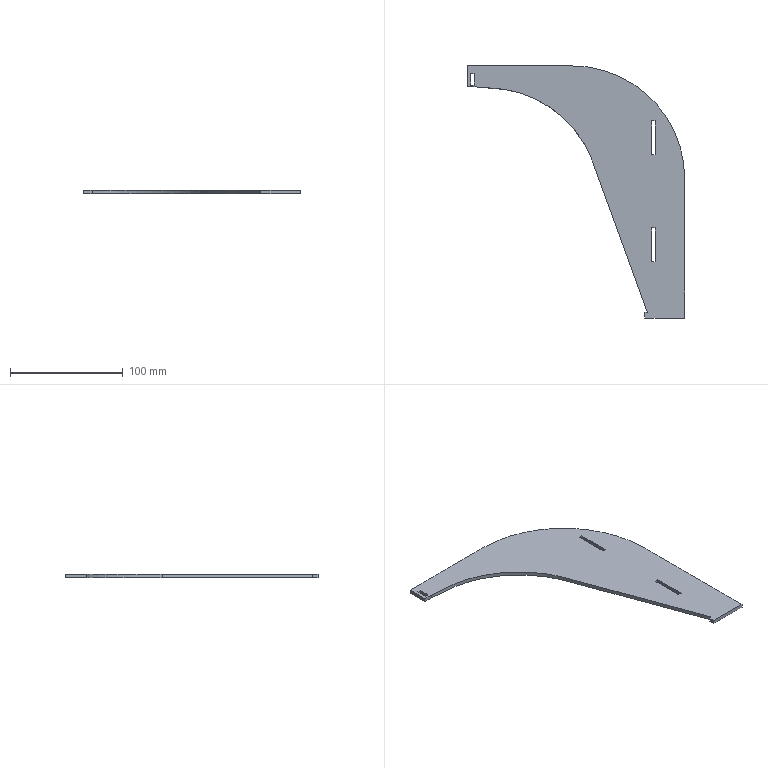Part | SolidWorks | features FlatPattern 1, SMBaseFlange 1, SheetMetal 1 | 1 solid | 24 faces | box 192.85 x 223.811 x 3.2 mm | volume 52018 mm3 | plane 22 | spline 1 | cylinder 1 | commonest cylinder face diameters 200 x1
STEP:
#1=CARTESIAN_POINT('',(111.323,-0.6438,0.));
#2=VERTEX_POINT('',#1);
#3=CARTESIAN_POINT('',(159.825,-133.885,0.));
#4=VERTEX_POINT('',#3);
#5=CARTESIAN_POINT('',(111.323,-0.6438,0.));
#6=CARTESIAN_POINT('',(127.491,-45.057,0.));
#7=CARTESIAN_POINT('',(143.658,-89.471,0.));
#8=CARTESIAN_POINT('',(159.825,-133.885,0.));
#9=B_SPLINE_CURVE_WITH_KNOTS('',3,(#5,#6,#7,#8),.UNSPECIFIED.,.F.,.F.,(4,4),(0.,1.),.UNSPECIFIED.);
#10=EDGE_CURVE('',#2,#4,#9,.T.);
#11=ORIENTED_EDGE('',*,*,#10,.F.);
#12=CARTESIAN_POINT('',(111.323,-0.6438,-3.2));
#13=VERTEX_POINT('',#12);
#14=CARTESIAN_POINT('',(111.323,-0.6438,-3.2));
#15=DIRECTION('',(0.,0.,1.));
#16=VECTOR('',#15,1000.);
#17=LINE('',#14,#16);
#18=EDGE_CURVE('',#13,#2,#17,.T.);
#19=ORIENTED_EDGE('',*,*,#18,.F.);
#20=CARTESIAN_POINT('',(159.825,-133.885,-3.2));
#21=VERTEX_POINT('',#20);
#22=CARTESIAN_POINT('',(111.323,-0.6438,-3.2));
#23=CARTESIAN_POINT('',(127.491,-45.057,-3.2));
#24=CARTESIAN_POINT('',(143.658,-89.471,-3.2));
#25=CARTESIAN_POINT('',(159.825,-133.885,-3.2));
#26=B_SPLINE_CURVE_WITH_KNOTS('',3,(#22,#23,#24,#25),.UNSPECIFIED.,.F.,.F.,(4,4),(0.,1.),.UNSPECIFIED.);
#27=EDGE_CURVE('',#13,#21,#26,.T.);
#28=ORIENTED_EDGE('',*,*,#27,.T.);
#29=CARTESIAN_POINT('',(159.825,-133.885,-3.2));
#30=DIRECTION('',(0.,0.,1.));
#31=VECTOR('',#30,1000.);
#32=LINE('',#29,#31);
#33=EDGE_CURVE('',#21,#4,#32,.T.);
#34=ORIENTED_EDGE('',*,*,#33,.T.);
#35=EDGE_LOOP('',(#11,#19,#28,#34));
#36=FACE_OUTER_BOUND('',#35,.T.);
#37=CARTESIAN_POINT('',(111.323,-0.6438,-3.2));
#38=DIRECTION('',(-0.9397,-0.3421,0.));
#39=DIRECTION('',(0.3421,-0.9397,0.));
#40=AXIS2_PLACEMENT_3D('',#37,#38,#39);
#41=PLANE('',#40);
#42=ADVANCED_FACE('',(#36),#41,.T.);
#43=CARTESIAN_POINT('',(7.851,66.042,0.));
#44=VERTEX_POINT('',#43);
#45=CARTESIAN_POINT('',(7.851,66.042,0.));
#46=CARTESIAN_POINT('',(9.365,65.953,0.));
#47=CARTESIAN_POINT('',(11.527,65.821,0.));
#48=CARTESIAN_POINT('',(13.859,65.666,0.));
#49=CARTESIAN_POINT('',(14.977,65.589,0.));
#50=CARTESIAN_POINT('',(15.525,65.55,0.));
#51=CARTESIAN_POINT('',(15.795,65.531,0.));
#52=CARTESIAN_POINT('',(15.93,65.521,0.));
#53=CARTESIAN_POINT('',(15.987,65.517,0.));
#54=CARTESIAN_POINT('',(16.026,65.514,0.));
#55=CARTESIAN_POINT('',(16.043,65.513,0.));
#56=CARTESIAN_POINT('',(17.399,65.415,0.));
#57=CARTESIAN_POINT('',(19.426,65.26,0.));
#58=CARTESIAN_POINT('',(21.833,65.063,0.));
#59=CARTESIAN_POINT('',(23.047,64.961,0.));
#60=CARTESIAN_POINT('',(23.657,64.908,0.));
#61=CARTESIAN_POINT('',(23.962,64.882,0.));
#62=CARTESIAN_POINT('',(24.115,64.868,0.));
#63=CARTESIAN_POINT('',(24.192,64.862,0.));
#64=CARTESIAN_POINT('',(24.23,64.858,0.));
#65=CARTESIAN_POINT('',(24.246,64.857,0.));
#66=CARTESIAN_POINT('',(24.257,64.856,0.));
#67=CARTESIAN_POINT('',(24.261,64.855,0.));
#68=CARTESIAN_POINT('',(25.155,64.777,0.));
#69=CARTESIAN_POINT('',(26.332,64.671,0.));
#70=CARTESIAN_POINT('',(27.438,64.563,0.));
#71=CARTESIAN_POINT('',(27.924,64.514,0.));
#72=CARTESIAN_POINT('',(28.15,64.49,0.));
#73=CARTESIAN_POINT('',(28.259,64.479,0.));
#74=CARTESIAN_POINT('',(28.312,64.473,0.));
#75=CARTESIAN_POINT('',(28.339,64.47,0.));
#76=CARTESIAN_POINT('',(28.35,64.469,0.));
#77=CARTESIAN_POINT('',(28.358,64.468,0.));
#78=CARTESIAN_POINT('',(28.36,64.468,0.));
#79=CARTESIAN_POINT('',(29.048,64.393,0.));
#80=CARTESIAN_POINT('',(30.071,64.272,0.));
#81=CARTESIAN_POINT('',(31.26,64.112,0.));
#82=CARTESIAN_POINT('',(31.769,64.039,0.));
#83=CARTESIAN_POINT('',(32.107,63.989,0.));
#84=CARTESIAN_POINT('',(32.276,63.964,0.));
#85=CARTESIAN_POINT('',(33.809,63.733,0.));
#86=CARTESIAN_POINT('',(35.841,63.383,0.));
#87=CARTESIAN_POINT('',(38.19,62.903,0.));
#88=CARTESIAN_POINT('',(39.192,62.682,0.));
#89=CARTESIAN_POINT('',(39.859,62.532,0.));
#90=CARTESIAN_POINT('',(40.19,62.455,0.));
#91=CARTESIAN_POINT('',(43.202,61.742,0.));
#92=CARTESIAN_POINT('',(45.843,61.001,0.));
#93=CARTESIAN_POINT('',(51.055,59.304,0.));
#94=CARTESIAN_POINT('',(53.626,58.346,0.));
#95=CARTESIAN_POINT('',(58.69,56.22,0.));
#96=CARTESIAN_POINT('',(62.412,54.473,0.));
#97=CARTESIAN_POINT('',(66.622,52.17,0.));
#98=CARTESIAN_POINT('',(68.397,51.126,0.));
#99=CARTESIAN_POINT('',(69.574,50.417,0.));
#100=CARTESIAN_POINT('',(70.161,50.056,0.));
#101=CARTESIAN_POINT('',(75.393,46.758,0.));
#102=CARTESIAN_POINT('',(79.774,43.464,0.));
#103=CARTESIAN_POINT('',(85.939,37.979,0.));
#104=CARTESIAN_POINT('',(87.911,36.073,0.));
#105=CARTESIAN_POINT('',(91.691,32.105,0.));
#106=CARTESIAN_POINT('',(93.498,30.044,0.));
#107=CARTESIAN_POINT('',(102.13,19.335,0.));
#108=CARTESIAN_POINT('',(107.496,9.82,0.));
#109=CARTESIAN_POINT('',(111.323,-0.6438,0.));
#110=B_SPLINE_CURVE_WITH_KNOTS('',3,(#45,#46,#47,#48,#49,#50,#51,#52,#53,#54,#55,#56,#57,#58,#59,#60,#61,#62,#63,#64,#65,#66,#67,#68,#69,#70,#71,#72,#73,#74,#75,#76,#77,#78,#79,#80,#81,#82,#83,#84,#85,#86,#87,#88,#89,#90,#91,#92,#93,#94,#95,#96,#97,#98,#99,#100,#101,#102,#103,#104,#105,#106,#107,#108,#109),.UNSPECIFIED.,.F.,.F.,(4,1,1,1,1,1,1,2,2,1,1,1,1,1,1,1,1,2,2,1,1,1,1,1,1,1,2,2,1,1,2,2,1,1,2,2,2,2,1,1,2,2,2,2,2,4),(0.,0.03125,0.04688,0.05469,0.05859,0.06055,0.06152,0.06201,0.0625,0.09375,0.1094,0.1172,0.1211,0.123,0.124,0.1245,0.1248,0.1249,0.125,0.1406,0.1484,0.1523,0.1543,0.1553,0.1558,0.156,0.1561,0.1563,0.1719,0.1797,0.1836,0.1875,0.2188,0.2344,0.2422,0.25,0.3125,0.375,0.4375,0.4688,0.4844,0.5,0.625,0.6875,0.75,1.),.UNSPECIFIED.);
#111=EDGE_CURVE('',#44,#2,#110,.T.);
#112=ORIENTED_EDGE('',*,*,#111,.F.);
#113=CARTESIAN_POINT('',(7.851,66.042,-3.2));
#114=VERTEX_POINT('',#113);
#115=CARTESIAN_POINT('',(7.851,66.042,-3.2));
#116=DIRECTION('',(0.,0.,1.));
#117=VECTOR('',#116,1000.);
#118=LINE('',#115,#117);
#119=EDGE_CURVE('',#114,#44,#118,.T.);
#120=ORIENTED_EDGE('',*,*,#119,.F.);
#121=CARTESIAN_POINT('',(7.851,66.042,-3.2));
#122=CARTESIAN_POINT('',(8.807,65.986,-3.2));
#123=CARTESIAN_POINT('',(10.707,65.875,-3.2));
#124=CARTESIAN_POINT('',(13.542,65.69,-3.2));
#125=CARTESIAN_POINT('',(16.343,65.493,-3.2));
#126=CARTESIAN_POINT('',(19.112,65.285,-3.2));
#127=CARTESIAN_POINT('',(21.849,65.065,-3.2));
#128=CARTESIAN_POINT('',(24.553,64.831,-3.2));
#129=CARTESIAN_POINT('',(27.228,64.593,-3.2));
#130=CARTESIAN_POINT('',(29.87,64.307,-3.2));
#131=CARTESIAN_POINT('',(32.473,63.946,-3.2));
#132=CARTESIAN_POINT('',(35.035,63.525,-3.2));
#133=CARTESIAN_POINT('',(37.554,63.043,-3.2));
#134=CARTESIAN_POINT('',(40.029,62.503,-3.2));
#135=CARTESIAN_POINT('',(42.458,61.909,-3.2));
#136=CARTESIAN_POINT('',(46.379,60.845,-3.2));
#137=CARTESIAN_POINT('',(50.928,59.371,-3.2));
#138=CARTESIAN_POINT('',(55.319,57.654,-3.2));
#139=CARTESIAN_POINT('',(58.804,56.148,-3.2));
#140=CARTESIAN_POINT('',(62.779,54.269,-3.2));
#141=CARTESIAN_POINT('',(67.787,51.558,-3.2));
#142=CARTESIAN_POINT('',(71.916,48.974,-3.2));
#143=CARTESIAN_POINT('',(74.698,47.071,-3.2));
#144=CARTESIAN_POINT('',(77.312,45.205,-3.2));
#145=CARTESIAN_POINT('',(81.211,42.191,-3.2));
#146=CARTESIAN_POINT('',(85.675,38.26,-3.2));
#147=CARTESIAN_POINT('',(88.926,35.024,-3.2));
#148=CARTESIAN_POINT('',(91.151,32.658,-3.2));
#149=CARTESIAN_POINT('',(93.506,30.029,-3.2));
#150=CARTESIAN_POINT('',(96.259,26.664,-3.2));
#151=CARTESIAN_POINT('',(99.436,22.362,-3.2));
#152=CARTESIAN_POINT('',(101.519,19.216,-3.2));
#153=CARTESIAN_POINT('',(103.337,16.242,-3.2));
#154=CARTESIAN_POINT('',(104.55,14.156,-3.2));
#155=CARTESIAN_POINT('',(106.188,11.13,-3.2));
#156=CARTESIAN_POINT('',(107.561,8.363,-3.2));
#157=CARTESIAN_POINT('',(108.775,5.705,-3.2));
#158=CARTESIAN_POINT('',(109.625,3.726,-3.2));
#159=CARTESIAN_POINT('',(110.339,1.96,-3.2));
#160=CARTESIAN_POINT('',(110.821,0.7113,-3.2));
#161=CARTESIAN_POINT('',(111.104,-0.04627,-3.2));
#162=CARTESIAN_POINT('',(111.244,-0.4271,-3.2));
#163=CARTESIAN_POINT('',(111.302,-0.5849,-3.2));
#164=CARTESIAN_POINT('',(111.323,-0.6438,-3.2));
#165=B_SPLINE_CURVE_WITH_KNOTS('',3,(#121,#122,#123,#124,#125,#126,#127,#128,#129,#130,#131,#132,#133,#134,#135,#136,#137,#138,#139,#140,#141,#142,#143,#144,#145,#146,#147,#148,#149,#150,#151,#152,#153,#154,#155,#156,#157,#158,#159,#160,#161,#162,#163,#164),.UNSPECIFIED.,.F.,.F.,(4,1,1,1,1,1,1,1,1,1,1,1,1,1,1,1,1,1,1,1,1,1,1,1,1,1,1,1,1,1,1,1,1,1,1,1,1,1,1,1,1,4),(0.,0.02181,0.04338,0.0647,0.08579,0.1066,0.1272,0.1476,0.1678,0.1878,0.2075,0.227,0.2462,0.2652,0.2839,0.3387,0.374,0.3913,0.4252,0.4742,0.521,0.5361,0.551,0.5942,0.6483,0.6864,0.6986,0.7223,0.7668,0.7976,0.8441,0.8527,0.877,0.8991,0.9311,0.9474,0.9657,0.9801,0.9908,0.9962,0.9986,1.),.UNSPECIFIED.);
#166=EDGE_CURVE('',#114,#13,#165,.T.);
#167=ORIENTED_EDGE('',*,*,#166,.T.);
#168=ORIENTED_EDGE('',*,*,#18,.T.);
#169=EDGE_LOOP('',(#112,#120,#167,#168));
#170=FACE_OUTER_BOUND('',#169,.T.);
#171=CARTESIAN_POINT('',(7.851,66.042,-3.2));
#172=CARTESIAN_POINT('',(7.851,66.042,0.));
#173=CARTESIAN_POINT('',(8.807,65.986,-3.2));
#174=CARTESIAN_POINT('',(8.807,65.986,0.));
#175=CARTESIAN_POINT('',(10.707,65.875,-3.2));
#176=CARTESIAN_POINT('',(10.707,65.875,0.));
#177=CARTESIAN_POINT('',(13.542,65.69,-3.2));
#178=CARTESIAN_POINT('',(13.542,65.69,0.));
#179=CARTESIAN_POINT('',(16.343,65.493,-3.2));
#180=CARTESIAN_POINT('',(16.343,65.493,0.));
#181=CARTESIAN_POINT('',(19.112,65.285,-3.2));
#182=CARTESIAN_POINT('',(19.112,65.285,0.));
#183=CARTESIAN_POINT('',(21.849,65.065,-3.2));
#184=CARTESIAN_POINT('',(21.849,65.065,0.));
#185=CARTESIAN_POINT('',(24.553,64.831,-3.2));
#186=CARTESIAN_POINT('',(24.553,64.831,0.));
#187=CARTESIAN_POINT('',(27.228,64.593,-3.2));
#188=CARTESIAN_POINT('',(27.228,64.593,0.));
#189=CARTESIAN_POINT('',(29.87,64.307,-3.2));
#190=CARTESIAN_POINT('',(29.87,64.307,0.));
#191=CARTESIAN_POINT('',(32.473,63.946,-3.2));
#192=CARTESIAN_POINT('',(32.473,63.946,0.));
#193=CARTESIAN_POINT('',(35.035,63.525,-3.2));
#194=CARTESIAN_POINT('',(35.035,63.525,0.));
#195=CARTESIAN_POINT('',(37.554,63.043,-3.2));
#196=CARTESIAN_POINT('',(37.554,63.043,0.));
#197=CARTESIAN_POINT('',(40.029,62.503,-3.2));
#198=CARTESIAN_POINT('',(40.029,62.503,0.));
#199=CARTESIAN_POINT('',(42.458,61.909,-3.2));
#200=CARTESIAN_POINT('',(42.458,61.909,0.));
#201=CARTESIAN_POINT('',(46.379,60.845,-3.2));
#202=CARTESIAN_POINT('',(46.379,60.845,0.));
#203=CARTESIAN_POINT('',(50.928,59.371,-3.2));
#204=CARTESIAN_POINT('',(50.928,59.371,0.));
#205=CARTESIAN_POINT('',(55.319,57.654,-3.2));
#206=CARTESIAN_POINT('',(55.319,57.654,0.));
#207=CARTESIAN_POINT('',(58.804,56.148,-3.2));
#208=CARTESIAN_POINT('',(58.804,56.148,0.));
#209=CARTESIAN_POINT('',(62.779,54.269,-3.2));
#210=CARTESIAN_POINT('',(62.779,54.269,0.));
#211=CARTESIAN_POINT('',(67.787,51.558,-3.2));
#212=CARTESIAN_POINT('',(67.787,51.558,0.));
#213=CARTESIAN_POINT('',(71.916,48.974,-3.2));
#214=CARTESIAN_POINT('',(71.916,48.974,0.));
#215=CARTESIAN_POINT('',(74.698,47.071,-3.2));
#216=CARTESIAN_POINT('',(74.698,47.071,0.));
#217=CARTESIAN_POINT('',(77.312,45.205,-3.2));
#218=CARTESIAN_POINT('',(77.312,45.205,0.));
#219=CARTESIAN_POINT('',(81.211,42.191,-3.2));
#220=CARTESIAN_POINT('',(81.211,42.191,0.));
#221=CARTESIAN_POINT('',(85.675,38.26,-3.2));
#222=CARTESIAN_POINT('',(85.675,38.26,0.));
#223=CARTESIAN_POINT('',(88.926,35.024,-3.2));
#224=CARTESIAN_POINT('',(88.926,35.024,0.));
#225=CARTESIAN_POINT('',(91.151,32.658,-3.2));
#226=CARTESIAN_POINT('',(91.151,32.658,0.));
#227=CARTESIAN_POINT('',(93.506,30.029,-3.2));
#228=CARTESIAN_POINT('',(93.506,30.029,0.));
#229=CARTESIAN_POINT('',(96.259,26.664,-3.2));
#230=CARTESIAN_POINT('',(96.259,26.664,0.));
#231=CARTESIAN_POINT('',(99.436,22.362,-3.2));
#232=CARTESIAN_POINT('',(99.436,22.362,0.));
#233=CARTESIAN_POINT('',(101.519,19.216,-3.2));
#234=CARTESIAN_POINT('',(101.519,19.216,0.));
#235=CARTESIAN_POINT('',(103.337,16.242,-3.2));
#236=CARTESIAN_POINT('',(103.337,16.242,0.));
#237=CARTESIAN_POINT('',(104.55,14.156,-3.2));
#238=CARTESIAN_POINT('',(104.55,14.156,0.));
#239=CARTESIAN_POINT('',(106.188,11.13,-3.2));
#240=CARTESIAN_POINT('',(106.188,11.13,0.));
#241=CARTESIAN_POINT('',(107.561,8.363,-3.2));
#242=CARTESIAN_POINT('',(107.561,8.363,0.));
#243=CARTESIAN_POINT('',(108.775,5.705,-3.2));
#244=CARTESIAN_POINT('',(108.775,5.705,0.));
#245=CARTESIAN_POINT('',(109.625,3.726,-3.2));
#246=CARTESIAN_POINT('',(109.625,3.726,0.));
#247=CARTESIAN_POINT('',(110.339,1.96,-3.2));
#248=CARTESIAN_POINT('',(110.339,1.96,0.));
#249=CARTESIAN_POINT('',(110.821,0.7113,-3.2));
#250=CARTESIAN_POINT('',(110.821,0.7113,0.));
#251=CARTESIAN_POINT('',(111.104,-0.04627,-3.2));
#252=CARTESIAN_POINT('',(111.104,-0.04627,0.));
#253=CARTESIAN_POINT('',(111.244,-0.4271,-3.2));
#254=CARTESIAN_POINT('',(111.244,-0.4271,0.));
#255=CARTESIAN_POINT('',(111.302,-0.5849,-3.2));
#256=CARTESIAN_POINT('',(111.302,-0.5849,0.));
#257=CARTESIAN_POINT('',(111.323,-0.6438,-3.2));
#258=CARTESIAN_POINT('',(111.323,-0.6438,0.));
#259=B_SPLINE_SURFACE_WITH_KNOTS('',3,1,((#171,#172),(#173,#174),(#175,#176),(#177,#178),(#179,#180),(#181,#182),(#183,#184),(#185,#186),(#187,#188),(#189,#190),(#191,#192),(#193,#194),(#195,#196),(#197,#198),(#199,#200),(#201,#202),(#203,#204),(#205,#206),(#207,#208),(#209,#210),(#211,#212),(#213,#214),(#215,#216),(#217,#218),(#219,#220),(#221,#222),(#223,#224),(#225,#226),(#227,#228),(#229,#230),(#231,#232),(#233,#234),(#235,#236),(#237,#238),(#239,#240),(#241,#242),(#243,#244),(#245,#246),(#247,#248),(#249,#250),(#251,#252),(#253,#254),(#255,#256),(#257,#258)),.UNSPECIFIED.,.F.,.F.,.F.,(4,1,1,1,1,1,1,1,1,1,1,1,1,1,1,1,1,1,1,1,1,1,1,1,1,1,1,1,1,1,1,1,1,1,1,1,1,1,1,1,1,4),(2,2),(0.,0.02181,0.04338,0.0647,0.08579,0.1066,0.1272,0.1476,0.1678,0.1878,0.2075,0.227,0.2462,0.2652,0.2839,0.3387,0.374,0.3913,0.4252,0.4742,0.521,0.5361,0.551,0.5942,0.6483,0.6864,0.6986,0.7223,0.7668,0.7976,0.8441,0.8527,0.877,0.8991,0.9311,0.9474,0.9657,0.9801,0.9908,0.9962,0.9986,1.),(0.,1.),.UNSPECIFIED.);
#260=ADVANCED_FACE('',(#170),#259,.T.);
#261=CARTESIAN_POINT('',(0.,66.042,0.));
#262=VERTEX_POINT('',#261);
#263=CARTESIAN_POINT('',(0.,66.042,0.));
#264=DIRECTION('',(1.,0.,0.));
#265=VECTOR('',#264,1000.);
#266=LINE('',#263,#265);
#267=EDGE_CURVE('',#262,#44,#266,.T.);
#268=ORIENTED_EDGE('',*,*,#267,.F.);
#269=CARTESIAN_POINT('',(0.,66.042,-3.2));
#270=VERTEX_POINT('',#269);
#271=CARTESIAN_POINT('',(0.,66.042,-3.2));
#272=DIRECTION('',(0.,0.,1.));
#273=VECTOR('',#272,1000.);
#274=LINE('',#271,#273);
#275=EDGE_CURVE('',#270,#262,#274,.T.);
#276=ORIENTED_EDGE('',*,*,#275,.F.);
#277=CARTESIAN_POINT('',(0.,66.042,-3.2));
#278=DIRECTION('',(1.,0.,0.));
#279=VECTOR('',#278,1000.);
#280=LINE('',#277,#279);
#281=EDGE_CURVE('',#270,#114,#280,.T.);
#282=ORIENTED_EDGE('',*,*,#281,.T.);
#283=ORIENTED_EDGE('',*,*,#119,.T.);
#284=EDGE_LOOP('',(#268,#276,#282,#283));
#285=FACE_OUTER_BOUND('',#284,.T.);
#286=CARTESIAN_POINT('',(0.,66.042,-3.2));
#287=DIRECTION('',(0.,-1.,0.));
#288=DIRECTION('',(0.,0.,-1.));
#289=AXIS2_PLACEMENT_3D('',#286,#287,#288);
#290=PLANE('',#289);
#291=ADVANCED_FACE('',(#285),#290,.T.);
#292=CARTESIAN_POINT('',(0.,84.724,0.));
#293=VERTEX_POINT('',#292);
#294=CARTESIAN_POINT('',(0.,84.724,0.));
#295=DIRECTION('',(0.,-1.,0.));
#296=VECTOR('',#295,1000.);
#297=LINE('',#294,#296);
#298=EDGE_CURVE('',#293,#262,#297,.T.);
#299=ORIENTED_EDGE('',*,*,#298,.F.);
#300=CARTESIAN_POINT('',(0.,84.724,-3.2));
#301=VERTEX_POINT('',#300);
#302=CARTESIAN_POINT('',(0.,84.724,-3.2));
#303=DIRECTION('',(0.,0.,1.));
#304=VECTOR('',#303,1000.);
#305=LINE('',#302,#304);
#306=EDGE_CURVE('',#301,#293,#305,.T.);
#307=ORIENTED_EDGE('',*,*,#306,.F.);
#308=CARTESIAN_POINT('',(0.,84.724,-3.2));
#309=DIRECTION('',(0.,-1.,0.));
#310=VECTOR('',#309,1000.);
#311=LINE('',#308,#310);
#312=EDGE_CURVE('',#301,#270,#311,.T.);
#313=ORIENTED_EDGE('',*,*,#312,.T.);
#314=ORIENTED_EDGE('',*,*,#275,.T.);
#315=EDGE_LOOP('',(#299,#307,#313,#314));
#316=FACE_OUTER_BOUND('',#315,.T.);
#317=CARTESIAN_POINT('',(0.,84.724,-3.2));
#318=DIRECTION('',(-1.,0.,0.));
#319=DIRECTION('',(0.,-1.,0.));
#320=AXIS2_PLACEMENT_3D('',#317,#318,#319);
#321=PLANE('',#320);
#322=ADVANCED_FACE('',(#316),#321,.T.);
#323=CARTESIAN_POINT('',(92.85,84.724,0.));
#324=VERTEX_POINT('',#323);
#325=CARTESIAN_POINT('',(0.,84.724,0.));
#326=DIRECTION('',(-1.,0.,0.));
#327=VECTOR('',#326,1000.);
#328=LINE('',#325,#327);
#329=EDGE_CURVE('',#324,#293,#328,.T.);
#330=ORIENTED_EDGE('',*,*,#329,.F.);
#331=CARTESIAN_POINT('',(92.85,84.724,-3.2));
#332=VERTEX_POINT('',#331);
#333=CARTESIAN_POINT('',(92.85,84.724,-3.2));
#334=DIRECTION('',(0.,0.,1.));
#335=VECTOR('',#334,1000.);
#336=LINE('',#333,#335);
#337=EDGE_CURVE('',#332,#324,#336,.T.);
#338=ORIENTED_EDGE('',*,*,#337,.F.);
#339=CARTESIAN_POINT('',(0.,84.724,-3.2));
#340=DIRECTION('',(-1.,0.,0.));
#341=VECTOR('',#340,1000.);
#342=LINE('',#339,#341);
#343=EDGE_CURVE('',#332,#301,#342,.T.);
#344=ORIENTED_EDGE('',*,*,#343,.T.);
#345=ORIENTED_EDGE('',*,*,#306,.T.);
#346=EDGE_LOOP('',(#330,#338,#344,#345));
#347=FACE_OUTER_BOUND('',#346,.T.);
#348=CARTESIAN_POINT('',(0.,84.724,-3.2));
#349=DIRECTION('',(0.,1.,0.));
#350=DIRECTION('',(-1.,0.,0.));
#351=AXIS2_PLACEMENT_3D('',#348,#349,#350);
#352=PLANE('',#351);
#353=ADVANCED_FACE('',(#347),#352,.T.);
#354=CARTESIAN_POINT('',(192.85,-15.276,0.));
#355=VERTEX_POINT('',#354);
#356=CARTESIAN_POINT('',(92.85,-15.276,0.));
#357=DIRECTION('',(0.,0.,1.));
#358=DIRECTION('',(-1.,0.,0.));
#359=AXIS2_PLACEMENT_3D('',#356,#357,#358);
#360=CIRCLE('',#359,100.);
#361=EDGE_CURVE('',#355,#324,#360,.T.);
#362=ORIENTED_EDGE('',*,*,#361,.F.);
#363=CARTESIAN_POINT('',(192.85,-15.276,-3.2));
#364=VERTEX_POINT('',#363);
#365=CARTESIAN_POINT('',(192.85,-15.276,-3.2));
#366=DIRECTION('',(0.,0.,1.));
#367=VECTOR('',#366,1000.);
#368=LINE('',#365,#367);
#369=EDGE_CURVE('',#364,#355,#368,.T.);
#370=ORIENTED_EDGE('',*,*,#369,.F.);
#371=CARTESIAN_POINT('',(92.85,-15.276,-3.2));
#372=DIRECTION('',(0.,0.,1.));
#373=DIRECTION('',(-1.,0.,0.));
#374=AXIS2_PLACEMENT_3D('',#371,#372,#373);
#375=CIRCLE('',#374,100.);
#376=EDGE_CURVE('',#364,#332,#375,.T.);
#377=ORIENTED_EDGE('',*,*,#376,.T.);
#378=ORIENTED_EDGE('',*,*,#337,.T.);
#379=EDGE_LOOP('',(#362,#370,#377,#378));
#380=FACE_OUTER_BOUND('',#379,.T.);
#381=CARTESIAN_POINT('',(92.85,-15.276,-3.2));
#382=DIRECTION('',(0.,0.,1.));
#383=DIRECTION('',(1.,0.,0.));
#384=AXIS2_PLACEMENT_3D('',#381,#382,#383);
#385=CYLINDRICAL_SURFACE('',#384,100.);
#386=ADVANCED_FACE('',(#380),#385,.T.);
#387=CARTESIAN_POINT('',(192.85,-139.086,0.));
#388=VERTEX_POINT('',#387);
#389=CARTESIAN_POINT('',(192.85,-15.276,0.));
#390=DIRECTION('',(0.,1.,0.));
#391=VECTOR('',#390,1000.);
#392=LINE('',#389,#391);
#393=EDGE_CURVE('',#388,#355,#392,.T.);
#394=ORIENTED_EDGE('',*,*,#393,.F.);
#395=CARTESIAN_POINT('',(192.85,-139.086,-3.2));
#396=VERTEX_POINT('',#395);
#397=CARTESIAN_POINT('',(192.85,-139.086,-3.2));
#398=DIRECTION('',(0.,0.,1.));
#399=VECTOR('',#398,1000.);
#400=LINE('',#397,#399);
#401=EDGE_CURVE('',#396,#388,#400,.T.);
#402=ORIENTED_EDGE('',*,*,#401,.F.);
#403=CARTESIAN_POINT('',(192.85,-15.276,-3.2));
#404=DIRECTION('',(0.,1.,0.));
#405=VECTOR('',#404,1000.);
#406=LINE('',#403,#405);
#407=EDGE_CURVE('',#396,#364,#406,.T.);
#408=ORIENTED_EDGE('',*,*,#407,.T.);
#409=ORIENTED_EDGE('',*,*,#369,.T.);
#410=EDGE_LOOP('',(#394,#402,#408,#409));
#411=FACE_OUTER_BOUND('',#410,.T.);
#412=CARTESIAN_POINT('',(192.85,-15.276,-3.2));
#413=DIRECTION('',(1.,0.,0.));
#414=DIRECTION('',(0.,1.,0.));
#415=AXIS2_PLACEMENT_3D('',#412,#413,#414);
#416=PLANE('',#415);
#417=ADVANCED_FACE('',(#411),#416,.T.);
#418=CARTESIAN_POINT('',(157.459,-139.086,0.));
#419=VERTEX_POINT('',#418);
#420=CARTESIAN_POINT('',(192.85,-139.086,0.));
#421=DIRECTION('',(1.,0.,0.));
#422=VECTOR('',#421,1000.);
#423=LINE('',#420,#422);
#424=EDGE_CURVE('',#419,#388,#423,.T.);
#425=ORIENTED_EDGE('',*,*,#424,.F.);
#426=CARTESIAN_POINT('',(157.459,-139.086,-3.2));
#427=VERTEX_POINT('',#426);
#428=CARTESIAN_POINT('',(157.459,-139.086,-3.2));
#429=DIRECTION('',(0.,0.,1.));
#430=VECTOR('',#429,1000.);
#431=LINE('',#428,#430);
#432=EDGE_CURVE('',#427,#419,#431,.T.);
#433=ORIENTED_EDGE('',*,*,#432,.F.);
#434=CARTESIAN_POINT('',(192.85,-139.086,-3.2));
#435=DIRECTION('',(1.,0.,0.));
#436=VECTOR('',#435,1000.);
#437=LINE('',#434,#436);
#438=EDGE_CURVE('',#427,#396,#437,.T.);
#439=ORIENTED_EDGE('',*,*,#438,.T.);
#440=ORIENTED_EDGE('',*,*,#401,.T.);
#441=EDGE_LOOP('',(#425,#433,#439,#440));
#442=FACE_OUTER_BOUND('',#441,.T.);
#443=CARTESIAN_POINT('',(192.85,-139.086,-3.2));
#444=DIRECTION('',(0.,-1.,0.));
#445=DIRECTION('',(0.,0.,-1.));
#446=AXIS2_PLACEMENT_3D('',#443,#444,#445);
#447=PLANE('',#446);
#448=ADVANCED_FACE('',(#442),#447,.T.);
#449=CARTESIAN_POINT('',(157.459,-134.086,0.));
#450=VERTEX_POINT('',#449);
#451=CARTESIAN_POINT('',(157.459,-139.086,0.));
#452=DIRECTION('',(0.,-1.,0.));
#453=VECTOR('',#452,1000.);
#454=LINE('',#451,#453);
#455=EDGE_CURVE('',#450,#419,#454,.T.);
#456=ORIENTED_EDGE('',*,*,#455,.F.);
#457=CARTESIAN_POINT('',(157.459,-134.086,-3.2));
#458=VERTEX_POINT('',#457);
#459=CARTESIAN_POINT('',(157.459,-134.086,-3.2));
#460=DIRECTION('',(0.,0.,1.));
#461=VECTOR('',#460,1000.);
#462=LINE('',#459,#461);
#463=EDGE_CURVE('',#458,#450,#462,.T.);
#464=ORIENTED_EDGE('',*,*,#463,.F.);
#465=CARTESIAN_POINT('',(157.459,-139.086,-3.2));
#466=DIRECTION('',(0.,-1.,0.));
#467=VECTOR('',#466,1000.);
#468=LINE('',#465,#467);
#469=EDGE_CURVE('',#458,#427,#468,.T.);
#470=ORIENTED_EDGE('',*,*,#469,.T.);
#471=ORIENTED_EDGE('',*,*,#432,.T.);
#472=EDGE_LOOP('',(#456,#464,#470,#471));
#473=FACE_OUTER_BOUND('',#472,.T.);
#474=CARTESIAN_POINT('',(157.459,-139.086,-3.2));
#475=DIRECTION('',(-1.,0.,0.));
#476=DIRECTION('',(0.,0.,1.));
#477=AXIS2_PLACEMENT_3D('',#474,#475,#476);
#478=PLANE('',#477);
#479=ADVANCED_FACE('',(#473),#478,.T.);
#480=CARTESIAN_POINT('',(157.459,-134.086,0.));
#481=DIRECTION('',(-0.9964,-0.08499,0.));
#482=VECTOR('',#481,1000.);
#483=LINE('',#480,#482);
#484=EDGE_CURVE('',#4,#450,#483,.T.);
#485=ORIENTED_EDGE('',*,*,#484,.F.);
#486=ORIENTED_EDGE('',*,*,#33,.F.);
#487=CARTESIAN_POINT('',(157.459,-134.086,-3.2));
#488=DIRECTION('',(-0.9964,-0.08499,0.));
#489=VECTOR('',#488,1000.);
#490=LINE('',#487,#489);
#491=EDGE_CURVE('',#21,#458,#490,.T.);
#492=ORIENTED_EDGE('',*,*,#491,.T.);
#493=ORIENTED_EDGE('',*,*,#463,.T.);
#494=EDGE_LOOP('',(#485,#486,#492,#493));
#495=FACE_OUTER_BOUND('',#494,.T.);
#496=CARTESIAN_POINT('',(157.459,-134.086,-3.2));
#497=DIRECTION('',(-0.08499,0.9964,0.));
#498=DIRECTION('',(-0.9964,-0.08499,0.));
#499=AXIS2_PLACEMENT_3D('',#496,#497,#498);
#500=PLANE('',#499);
#501=ADVANCED_FACE('',(#495),#500,.T.);
#502=CARTESIAN_POINT('',(166.708,-89.086,-3.2));
#503=VERTEX_POINT('',#502);
#504=CARTESIAN_POINT('',(166.708,-59.086,-3.2));
#505=VERTEX_POINT('',#504);
#506=CARTESIAN_POINT('',(166.708,-89.086,-3.2));
#507=DIRECTION('',(0.,1.,0.));
#508=VECTOR('',#507,1000.);
#509=LINE('',#506,#508);
#510=EDGE_CURVE('',#503,#505,#509,.T.);
#511=ORIENTED_EDGE('',*,*,#510,.T.);
#512=CARTESIAN_POINT('',(163.508,-59.086,-3.2));
#513=VERTEX_POINT('',#512);
#514=CARTESIAN_POINT('',(166.708,-59.086,-3.2));
#515=DIRECTION('',(-1.,0.,0.));
#516=VECTOR('',#515,1000.);
#517=LINE('',#514,#516);
#518=EDGE_CURVE('',#505,#513,#517,.T.);
#519=ORIENTED_EDGE('',*,*,#518,.T.);
#520=CARTESIAN_POINT('',(163.508,-89.086,-3.2));
#521=VERTEX_POINT('',#520);
#522=CARTESIAN_POINT('',(163.508,-89.086,-3.2));
#523=DIRECTION('',(0.,-1.,0.));
#524=VECTOR('',#523,1000.);
#525=LINE('',#522,#524);
#526=EDGE_CURVE('',#513,#521,#525,.T.);
#527=ORIENTED_EDGE('',*,*,#526,.T.);
#528=CARTESIAN_POINT('',(166.708,-89.086,-3.2));
#529=DIRECTION('',(1.,0.,0.));
#530=VECTOR('',#529,1000.);
#531=LINE('',#528,#530);
#532=EDGE_CURVE('',#521,#503,#531,.T.);
#533=ORIENTED_EDGE('',*,*,#532,.T.);
#534=EDGE_LOOP('',(#511,#519,#527,#533));
#535=FACE_BOUND('',#534,.T.);
#536=CARTESIAN_POINT('',(163.508,35.914,-3.2));
#537=VERTEX_POINT('',#536);
#538=CARTESIAN_POINT('',(163.508,5.914,-3.2));
#539=VERTEX_POINT('',#538);
#540=CARTESIAN_POINT('',(163.508,35.914,-3.2));
#541=DIRECTION('',(0.,-1.,0.));
#542=VECTOR('',#541,1000.);
#543=LINE('',#540,#542);
#544=EDGE_CURVE('',#537,#539,#543,.T.);
#545=ORIENTED_EDGE('',*,*,#544,.T.);
#546=CARTESIAN_POINT('',(166.708,5.914,-3.2));
#547=VERTEX_POINT('',#546);
#548=CARTESIAN_POINT('',(163.508,5.914,-3.2));
#549=DIRECTION('',(1.,0.,0.));
#550=VECTOR('',#549,1000.);
#551=LINE('',#548,#550);
#552=EDGE_CURVE('',#539,#547,#551,.T.);
#553=ORIENTED_EDGE('',*,*,#552,.T.);
#554=CARTESIAN_POINT('',(166.708,35.914,-3.2));
#555=VERTEX_POINT('',#554);
#556=CARTESIAN_POINT('',(166.708,35.914,-3.2));
#557=DIRECTION('',(0.,1.,0.));
#558=VECTOR('',#557,1000.);
#559=LINE('',#556,#558);
#560=EDGE_CURVE('',#547,#555,#559,.T.);
#561=ORIENTED_EDGE('',*,*,#560,.T.);
#562=CARTESIAN_POINT('',(163.508,35.914,-3.2));
#563=DIRECTION('',(-1.,0.,0.));
#564=VECTOR('',#563,1000.);
#565=LINE('',#562,#564);
#566=EDGE_CURVE('',#555,#537,#565,.T.);
#567=ORIENTED_EDGE('',*,*,#566,.T.);
#568=EDGE_LOOP('',(#545,#553,#561,#567));
#569=FACE_BOUND('',#568,.T.);
#570=CARTESIAN_POINT('',(2.85,77.724,-3.2));
#571=VERTEX_POINT('',#570);
#572=CARTESIAN_POINT('',(2.85,67.724,-3.2));
#573=VERTEX_POINT('',#572);
#574=CARTESIAN_POINT('',(2.85,77.724,-3.2));
#575=DIRECTION('',(0.,-1.,0.));
#576=VECTOR('',#575,1000.);
#577=LINE('',#574,#576);
#578=EDGE_CURVE('',#571,#573,#577,.T.);
#579=ORIENTED_EDGE('',*,*,#578,.T.);
#580=CARTESIAN_POINT('',(6.05,67.724,-3.2));
#581=VERTEX_POINT('',#580);
#582=CARTESIAN_POINT('',(2.85,67.724,-3.2));
#583=DIRECTION('',(1.,0.,0.));
#584=VECTOR('',#583,1000.);
#585=LINE('',#582,#584);
#586=EDGE_CURVE('',#573,#581,#585,.T.);
#587=ORIENTED_EDGE('',*,*,#586,.T.);
#588=CARTESIAN_POINT('',(6.05,77.724,-3.2));
#589=VERTEX_POINT('',#588);
#590=CARTESIAN_POINT('',(6.05,77.724,-3.2));
#591=DIRECTION('',(0.,1.,0.));
#592=VECTOR('',#591,1000.);
#593=LINE('',#590,#592);
#594=EDGE_CURVE('',#581,#589,#593,.T.);
#595=ORIENTED_EDGE('',*,*,#594,.T.);
#596=CARTESIAN_POINT('',(2.85,77.724,-3.2));
#597=DIRECTION('',(-1.,0.,0.));
#598=VECTOR('',#597,1000.);
#599=LINE('',#596,#598);
#600=EDGE_CURVE('',#589,#571,#599,.T.);
#601=ORIENTED_EDGE('',*,*,#600,.T.);
#602=EDGE_LOOP('',(#579,#587,#595,#601));
#603=FACE_BOUND('',#602,.T.);
#604=ORIENTED_EDGE('',*,*,#27,.F.);
#605=ORIENTED_EDGE('',*,*,#166,.F.);
#606=ORIENTED_EDGE('',*,*,#281,.F.);
#607=ORIENTED_EDGE('',*,*,#312,.F.);
#608=ORIENTED_EDGE('',*,*,#343,.F.);
#609=ORIENTED_EDGE('',*,*,#376,.F.);
#610=ORIENTED_EDGE('',*,*,#407,.F.);
#611=ORIENTED_EDGE('',*,*,#438,.F.);
#612=ORIENTED_EDGE('',*,*,#469,.F.);
#613=ORIENTED_EDGE('',*,*,#491,.F.);
#614=EDGE_LOOP('',(#604,#605,#606,#607,#608,#609,#610,#611,#612,#613));
#615=FACE_OUTER_BOUND('',#614,.T.);
#616=CARTESIAN_POINT('',(92.85,-15.276,-3.2));
#617=DIRECTION('',(0.,0.,-1.));
#618=DIRECTION('',(-1.,0.,0.));
#619=AXIS2_PLACEMENT_3D('',#616,#617,#618);
#620=PLANE('',#619);
#621=ADVANCED_FACE('',(#535,#569,#603,#615),#620,.T.);
#622=CARTESIAN_POINT('',(166.708,-59.086,0.));
#623=VERTEX_POINT('',#622);
#624=CARTESIAN_POINT('',(163.508,-59.086,0.));
#625=VERTEX_POINT('',#624);
#626=CARTESIAN_POINT('',(166.708,-59.086,0.));
#627=DIRECTION('',(-1.,0.,0.));
#628=VECTOR('',#627,1000.);
#629=LINE('',#626,#628);
#630=EDGE_CURVE('',#623,#625,#629,.T.);
#631=ORIENTED_EDGE('',*,*,#630,.F.);
#632=CARTESIAN_POINT('',(166.708,-89.086,0.));
#633=VERTEX_POINT('',#632);
#634=CARTESIAN_POINT('',(166.708,-89.086,0.));
#635=DIRECTION('',(0.,1.,0.));
#636=VECTOR('',#635,1000.);
#637=LINE('',#634,#636);
#638=EDGE_CURVE('',#633,#623,#637,.T.);
#639=ORIENTED_EDGE('',*,*,#638,.F.);
#640=CARTESIAN_POINT('',(163.508,-89.086,0.));
#641=VERTEX_POINT('',#640);
#642=CARTESIAN_POINT('',(166.708,-89.086,0.));
#643=DIRECTION('',(1.,0.,0.));
#644=VECTOR('',#643,1000.);
#645=LINE('',#642,#644);
#646=EDGE_CURVE('',#641,#633,#645,.T.);
#647=ORIENTED_EDGE('',*,*,#646,.F.);
#648=CARTESIAN_POINT('',(163.508,-89.086,0.));
#649=DIRECTION('',(0.,-1.,0.));
#650=VECTOR('',#649,1000.);
#651=LINE('',#648,#650);
#652=EDGE_CURVE('',#625,#641,#651,.T.);
#653=ORIENTED_EDGE('',*,*,#652,.F.);
#654=EDGE_LOOP('',(#631,#639,#647,#653));
#655=FACE_BOUND('',#654,.T.);
#656=CARTESIAN_POINT('',(163.508,5.914,0.));
#657=VERTEX_POINT('',#656);
#658=CARTESIAN_POINT('',(166.708,5.914,0.));
#659=VERTEX_POINT('',#658);
#660=CARTESIAN_POINT('',(163.508,5.914,0.));
#661=DIRECTION('',(1.,0.,0.));
#662=VECTOR('',#661,1000.);
#663=LINE('',#660,#662);
#664=EDGE_CURVE('',#657,#659,#663,.T.);
#665=ORIENTED_EDGE('',*,*,#664,.F.);
#666=CARTESIAN_POINT('',(163.508,35.914,0.));
#667=VERTEX_POINT('',#666);
#668=CARTESIAN_POINT('',(163.508,35.914,0.));
#669=DIRECTION('',(0.,-1.,0.));
#670=VECTOR('',#669,1000.);
#671=LINE('',#668,#670);
#672=EDGE_CURVE('',#667,#657,#671,.T.);
#673=ORIENTED_EDGE('',*,*,#672,.F.);
#674=CARTESIAN_POINT('',(166.708,35.914,0.));
#675=VERTEX_POINT('',#674);
#676=CARTESIAN_POINT('',(163.508,35.914,0.));
#677=DIRECTION('',(-1.,0.,0.));
#678=VECTOR('',#677,1000.);
#679=LINE('',#676,#678);
#680=EDGE_CURVE('',#675,#667,#679,.T.);
#681=ORIENTED_EDGE('',*,*,#680,.F.);
#682=CARTESIAN_POINT('',(166.708,35.914,0.));
#683=DIRECTION('',(0.,1.,0.));
#684=VECTOR('',#683,1000.);
#685=LINE('',#682,#684);
#686=EDGE_CURVE('',#659,#675,#685,.T.);
#687=ORIENTED_EDGE('',*,*,#686,.F.);
#688=EDGE_LOOP('',(#665,#673,#681,#687));
#689=FACE_BOUND('',#688,.T.);
#690=CARTESIAN_POINT('',(2.85,67.724,0.));
#691=VERTEX_POINT('',#690);
#692=CARTESIAN_POINT('',(6.05,67.724,0.));
#693=VERTEX_POINT('',#692);
#694=CARTESIAN_POINT('',(2.85,67.724,0.));
#695=DIRECTION('',(1.,0.,0.));
#696=VECTOR('',#695,1000.);
#697=LINE('',#694,#696);
#698=EDGE_CURVE('',#691,#693,#697,.T.);
#699=ORIENTED_EDGE('',*,*,#698,.F.);
#700=CARTESIAN_POINT('',(2.85,77.724,0.));
#701=VERTEX_POINT('',#700);
#702=CARTESIAN_POINT('',(2.85,77.724,0.));
#703=DIRECTION('',(0.,-1.,0.));
#704=VECTOR('',#703,1000.);
#705=LINE('',#702,#704);
#706=EDGE_CURVE('',#701,#691,#705,.T.);
#707=ORIENTED_EDGE('',*,*,#706,.F.);
#708=CARTESIAN_POINT('',(6.05,77.724,0.));
#709=VERTEX_POINT('',#708);
#710=CARTESIAN_POINT('',(2.85,77.724,0.));
#711=DIRECTION('',(-1.,0.,0.));
#712=VECTOR('',#711,1000.);
#713=LINE('',#710,#712);
#714=EDGE_CURVE('',#709,#701,#713,.T.);
#715=ORIENTED_EDGE('',*,*,#714,.F.);
#716=CARTESIAN_POINT('',(6.05,77.724,0.));
#717=DIRECTION('',(0.,1.,0.));
#718=VECTOR('',#717,1000.);
#719=LINE('',#716,#718);
#720=EDGE_CURVE('',#693,#709,#719,.T.);
#721=ORIENTED_EDGE('',*,*,#720,.F.);
#722=EDGE_LOOP('',(#699,#707,#715,#721));
#723=FACE_BOUND('',#722,.T.);
#724=ORIENTED_EDGE('',*,*,#10,.T.);
#725=ORIENTED_EDGE('',*,*,#484,.T.);
#726=ORIENTED_EDGE('',*,*,#455,.T.);
#727=ORIENTED_EDGE('',*,*,#424,.T.);
#728=ORIENTED_EDGE('',*,*,#393,.T.);
#729=ORIENTED_EDGE('',*,*,#361,.T.);
#730=ORIENTED_EDGE('',*,*,#329,.T.);
#731=ORIENTED_EDGE('',*,*,#298,.T.);
#732=ORIENTED_EDGE('',*,*,#267,.T.);
#733=ORIENTED_EDGE('',*,*,#111,.T.);
#734=EDGE_LOOP('',(#724,#725,#726,#727,#728,#729,#730,#731,#732,#733));
#735=FACE_OUTER_BOUND('',#734,.T.);
#736=CARTESIAN_POINT('',(92.85,-15.276,0.));
#737=DIRECTION('',(0.,0.,-1.));
#738=DIRECTION('',(-1.,0.,0.));
#739=AXIS2_PLACEMENT_3D('',#736,#737,#738);
#740=PLANE('',#739);
#741=ADVANCED_FACE('',(#655,#689,#723,#735),#740,.F.);
#742=ORIENTED_EDGE('',*,*,#706,.T.);
#743=CARTESIAN_POINT('',(2.85,67.724,-3.2));
#744=DIRECTION('',(0.,0.,1.));
#745=VECTOR('',#744,1000.);
#746=LINE('',#743,#745);
#747=EDGE_CURVE('',#573,#691,#746,.T.);
#748=ORIENTED_EDGE('',*,*,#747,.F.);
#749=ORIENTED_EDGE('',*,*,#578,.F.);
#750=CARTESIAN_POINT('',(2.85,77.724,-3.2));
#751=DIRECTION('',(0.,0.,1.));
#752=VECTOR('',#751,1000.);
#753=LINE('',#750,#752);
#754=EDGE_CURVE('',#571,#701,#753,.T.);
#755=ORIENTED_EDGE('',*,*,#754,.T.);
#756=EDGE_LOOP('',(#742,#748,#749,#755));
#757=FACE_OUTER_BOUND('',#756,.T.);
#758=CARTESIAN_POINT('',(2.85,77.724,-3.2));
#759=DIRECTION('',(-1.,0.,0.));
#760=DIRECTION('',(0.,-1.,0.));
#761=AXIS2_PLACEMENT_3D('',#758,#759,#760);
#762=PLANE('',#761);
#763=ADVANCED_FACE('',(#757),#762,.F.);
#764=ORIENTED_EDGE('',*,*,#714,.T.);
#765=ORIENTED_EDGE('',*,*,#754,.F.);
#766=ORIENTED_EDGE('',*,*,#600,.F.);
#767=CARTESIAN_POINT('',(6.05,77.724,-3.2));
#768=DIRECTION('',(0.,0.,1.));
#769=VECTOR('',#768,1000.);
#770=LINE('',#767,#769);
#771=EDGE_CURVE('',#589,#709,#770,.T.);
#772=ORIENTED_EDGE('',*,*,#771,.T.);
#773=EDGE_LOOP('',(#764,#765,#766,#772));
#774=FACE_OUTER_BOUND('',#773,.T.);
#775=CARTESIAN_POINT('',(2.85,77.724,-3.2));
#776=DIRECTION('',(0.,1.,0.));
#777=DIRECTION('',(0.,0.,1.));
#778=AXIS2_PLACEMENT_3D('',#775,#776,#777);
#779=PLANE('',#778);
#780=ADVANCED_FACE('',(#774),#779,.F.);
#781=ORIENTED_EDGE('',*,*,#720,.T.);
#782=ORIENTED_EDGE('',*,*,#771,.F.);
#783=ORIENTED_EDGE('',*,*,#594,.F.);
#784=CARTESIAN_POINT('',(6.05,67.724,-3.2));
#785=DIRECTION('',(0.,0.,1.));
#786=VECTOR('',#785,1000.);
#787=LINE('',#784,#786);
#788=EDGE_CURVE('',#581,#693,#787,.T.);
#789=ORIENTED_EDGE('',*,*,#788,.T.);
#790=EDGE_LOOP('',(#781,#782,#783,#789));
#791=FACE_OUTER_BOUND('',#790,.T.);
#792=CARTESIAN_POINT('',(6.05,77.724,-3.2));
#793=DIRECTION('',(1.,0.,0.));
#794=DIRECTION('',(0.,1.,0.));
#795=AXIS2_PLACEMENT_3D('',#792,#793,#794);
#796=PLANE('',#795);
#797=ADVANCED_FACE('',(#791),#796,.F.);
#798=ORIENTED_EDGE('',*,*,#698,.T.);
#799=ORIENTED_EDGE('',*,*,#788,.F.);
#800=ORIENTED_EDGE('',*,*,#586,.F.);
#801=ORIENTED_EDGE('',*,*,#747,.T.);
#802=EDGE_LOOP('',(#798,#799,#800,#801));
#803=FACE_OUTER_BOUND('',#802,.T.);
#804=CARTESIAN_POINT('',(2.85,67.724,-3.2));
#805=DIRECTION('',(0.,-1.,0.));
#806=DIRECTION('',(0.,0.,-1.));
#807=AXIS2_PLACEMENT_3D('',#804,#805,#806);
#808=PLANE('',#807);
#809=ADVANCED_FACE('',(#803),#808,.F.);
#810=ORIENTED_EDGE('',*,*,#672,.T.);
#811=CARTESIAN_POINT('',(163.508,5.914,-3.2));
#812=DIRECTION('',(0.,0.,1.));
#813=VECTOR('',#812,1000.);
#814=LINE('',#811,#813);
#815=EDGE_CURVE('',#539,#657,#814,.T.);
#816=ORIENTED_EDGE('',*,*,#815,.F.);
#817=ORIENTED_EDGE('',*,*,#544,.F.);
#818=CARTESIAN_POINT('',(163.508,35.914,-3.2));
#819=DIRECTION('',(0.,0.,1.));
#820=VECTOR('',#819,1000.);
#821=LINE('',#818,#820);
#822=EDGE_CURVE('',#537,#667,#821,.T.);
#823=ORIENTED_EDGE('',*,*,#822,.T.);
#824=EDGE_LOOP('',(#810,#816,#817,#823));
#825=FACE_OUTER_BOUND('',#824,.T.);
#826=CARTESIAN_POINT('',(163.508,35.914,-3.2));
#827=DIRECTION('',(-1.,0.,0.));
#828=DIRECTION('',(0.,0.,1.));
#829=AXIS2_PLACEMENT_3D('',#826,#827,#828);
#830=PLANE('',#829);
#831=ADVANCED_FACE('',(#825),#830,.F.);
#832=ORIENTED_EDGE('',*,*,#680,.T.);
#833=ORIENTED_EDGE('',*,*,#822,.F.);
#834=ORIENTED_EDGE('',*,*,#566,.F.);
#835=CARTESIAN_POINT('',(166.708,35.914,-3.2));
#836=DIRECTION('',(0.,0.,1.));
#837=VECTOR('',#836,1000.);
#838=LINE('',#835,#837);
#839=EDGE_CURVE('',#555,#675,#838,.T.);
#840=ORIENTED_EDGE('',*,*,#839,.T.);
#841=EDGE_LOOP('',(#832,#833,#834,#840));
#842=FACE_OUTER_BOUND('',#841,.T.);
#843=CARTESIAN_POINT('',(163.508,35.914,-3.2));
#844=DIRECTION('',(0.,1.,0.));
#845=DIRECTION('',(0.,0.,1.));
#846=AXIS2_PLACEMENT_3D('',#843,#844,#845);
#847=PLANE('',#846);
#848=ADVANCED_FACE('',(#842),#847,.F.);
#849=ORIENTED_EDGE('',*,*,#686,.T.);
#850=ORIENTED_EDGE('',*,*,#839,.F.);
#851=ORIENTED_EDGE('',*,*,#560,.F.);
#852=CARTESIAN_POINT('',(166.708,5.914,-3.2));
#853=DIRECTION('',(0.,0.,1.));
#854=VECTOR('',#853,1000.);
#855=LINE('',#852,#854);
#856=EDGE_CURVE('',#547,#659,#855,.T.);
#857=ORIENTED_EDGE('',*,*,#856,.T.);
#858=EDGE_LOOP('',(#849,#850,#851,#857));
#859=FACE_OUTER_BOUND('',#858,.T.);
#860=CARTESIAN_POINT('',(166.708,35.914,-3.2));
#861=DIRECTION('',(1.,0.,0.));
#862=DIRECTION('',(0.,0.,-1.));
#863=AXIS2_PLACEMENT_3D('',#860,#861,#862);
#864=PLANE('',#863);
#865=ADVANCED_FACE('',(#859),#864,.F.);
#866=ORIENTED_EDGE('',*,*,#664,.T.);
#867=ORIENTED_EDGE('',*,*,#856,.F.);
#868=ORIENTED_EDGE('',*,*,#552,.F.);
#869=ORIENTED_EDGE('',*,*,#815,.T.);
#870=EDGE_LOOP('',(#866,#867,#868,#869));
#871=FACE_OUTER_BOUND('',#870,.T.);
#872=CARTESIAN_POINT('',(163.508,5.914,-3.2));
#873=DIRECTION('',(0.,-1.,0.));
#874=DIRECTION('',(0.,0.,-1.));
#875=AXIS2_PLACEMENT_3D('',#872,#873,#874);
#876=PLANE('',#875);
#877=ADVANCED_FACE('',(#871),#876,.F.);
#878=ORIENTED_EDGE('',*,*,#638,.T.);
#879=CARTESIAN_POINT('',(166.708,-59.086,-3.2));
#880=DIRECTION('',(0.,0.,1.));
#881=VECTOR('',#880,1000.);
#882=LINE('',#879,#881);
#883=EDGE_CURVE('',#505,#623,#882,.T.);
#884=ORIENTED_EDGE('',*,*,#883,.F.);
#885=ORIENTED_EDGE('',*,*,#510,.F.);
#886=CARTESIAN_POINT('',(166.708,-89.086,-3.2));
#887=DIRECTION('',(0.,0.,1.));
#888=VECTOR('',#887,1000.);
#889=LINE('',#886,#888);
#890=EDGE_CURVE('',#503,#633,#889,.T.);
#891=ORIENTED_EDGE('',*,*,#890,.T.);
#892=EDGE_LOOP('',(#878,#884,#885,#891));
#893=FACE_OUTER_BOUND('',#892,.T.);
#894=CARTESIAN_POINT('',(166.708,-89.086,-3.2));
#895=DIRECTION('',(1.,0.,0.));
#896=DIRECTION('',(0.,0.,-1.));
#897=AXIS2_PLACEMENT_3D('',#894,#895,#896);
#898=PLANE('',#897);
#899=ADVANCED_FACE('',(#893),#898,.F.);
#900=ORIENTED_EDGE('',*,*,#646,.T.);
#901=ORIENTED_EDGE('',*,*,#890,.F.);
#902=ORIENTED_EDGE('',*,*,#532,.F.);
#903=CARTESIAN_POINT('',(163.508,-89.086,-3.2));
#904=DIRECTION('',(0.,0.,1.));
#905=VECTOR('',#904,1000.);
#906=LINE('',#903,#905);
#907=EDGE_CURVE('',#521,#641,#906,.T.);
#908=ORIENTED_EDGE('',*,*,#907,.T.);
#909=EDGE_LOOP('',(#900,#901,#902,#908));
#910=FACE_OUTER_BOUND('',#909,.T.);
#911=CARTESIAN_POINT('',(166.708,-89.086,-3.2));
#912=DIRECTION('',(0.,-1.,0.));
#913=DIRECTION('',(0.,0.,-1.));
#914=AXIS2_PLACEMENT_3D('',#911,#912,#913);
#915=PLANE('',#914);
#916=ADVANCED_FACE('',(#910),#915,.F.);
#917=ORIENTED_EDGE('',*,*,#652,.T.);
#918=ORIENTED_EDGE('',*,*,#907,.F.);
#919=ORIENTED_EDGE('',*,*,#526,.F.);
#920=CARTESIAN_POINT('',(163.508,-59.086,-3.2));
#921=DIRECTION('',(0.,0.,1.));
#922=VECTOR('',#921,1000.);
#923=LINE('',#920,#922);
#924=EDGE_CURVE('',#513,#625,#923,.T.);
#925=ORIENTED_EDGE('',*,*,#924,.T.);
#926=EDGE_LOOP('',(#917,#918,#919,#925));
#927=FACE_OUTER_BOUND('',#926,.T.);
#928=CARTESIAN_POINT('',(163.508,-89.086,-3.2));
#929=DIRECTION('',(-1.,0.,0.));
#930=DIRECTION('',(0.,0.,1.));
#931=AXIS2_PLACEMENT_3D('',#928,#929,#930);
#932=PLANE('',#931);
#933=ADVANCED_FACE('',(#927),#932,.F.);
#934=ORIENTED_EDGE('',*,*,#630,.T.);
#935=ORIENTED_EDGE('',*,*,#924,.F.);
#936=ORIENTED_EDGE('',*,*,#518,.F.);
#937=ORIENTED_EDGE('',*,*,#883,.T.);
#938=EDGE_LOOP('',(#934,#935,#936,#937));
#939=FACE_OUTER_BOUND('',#938,.T.);
#940=CARTESIAN_POINT('',(166.708,-59.086,-3.2));
#941=DIRECTION('',(0.,1.,0.));
#942=DIRECTION('',(0.,0.,1.));
#943=AXIS2_PLACEMENT_3D('',#940,#941,#942);
#944=PLANE('',#943);
#945=ADVANCED_FACE('',(#939),#944,.F.);
#946=CLOSED_SHELL('',(#42,#260,#291,#322,#353,#386,#417,#448,#479,#501,#621,#741,#763,#780,#797,#809,#831,#848,#865,#877,#899,#916,#933,#945));
#947=MANIFOLD_SOLID_BREP('',#946);
#948=CARTESIAN_POINT('',(0.,0.,0.));
#949=DIRECTION('',(0.,0.,1.));
#950=DIRECTION('',(1.,0.,0.));
#951=AXIS2_PLACEMENT_3D('',#948,#949,#950);
#952=(LENGTH_UNIT()NAMED_UNIT(*)SI_UNIT(.MILLI.,.METRE.));
#953=UNCERTAINTY_MEASURE_WITH_UNIT(LENGTH_MEASURE(0.00001),#952,'','');
#954=(NAMED_UNIT(*)PLANE_ANGLE_UNIT()SI_UNIT($,.RADIAN.));
#955=(NAMED_UNIT(*)SI_UNIT($,.STERADIAN.)SOLID_ANGLE_UNIT());
#956=(GEOMETRIC_REPRESENTATION_CONTEXT(3)GLOBAL_UNCERTAINTY_ASSIGNED_CONTEXT((#953))GLOBAL_UNIT_ASSIGNED_CONTEXT((#952,#954,#955))REPRESENTATION_CONTEXT('',''));
#957=ADVANCED_BREP_SHAPE_REPRESENTATION('',(#947,#951),#956);